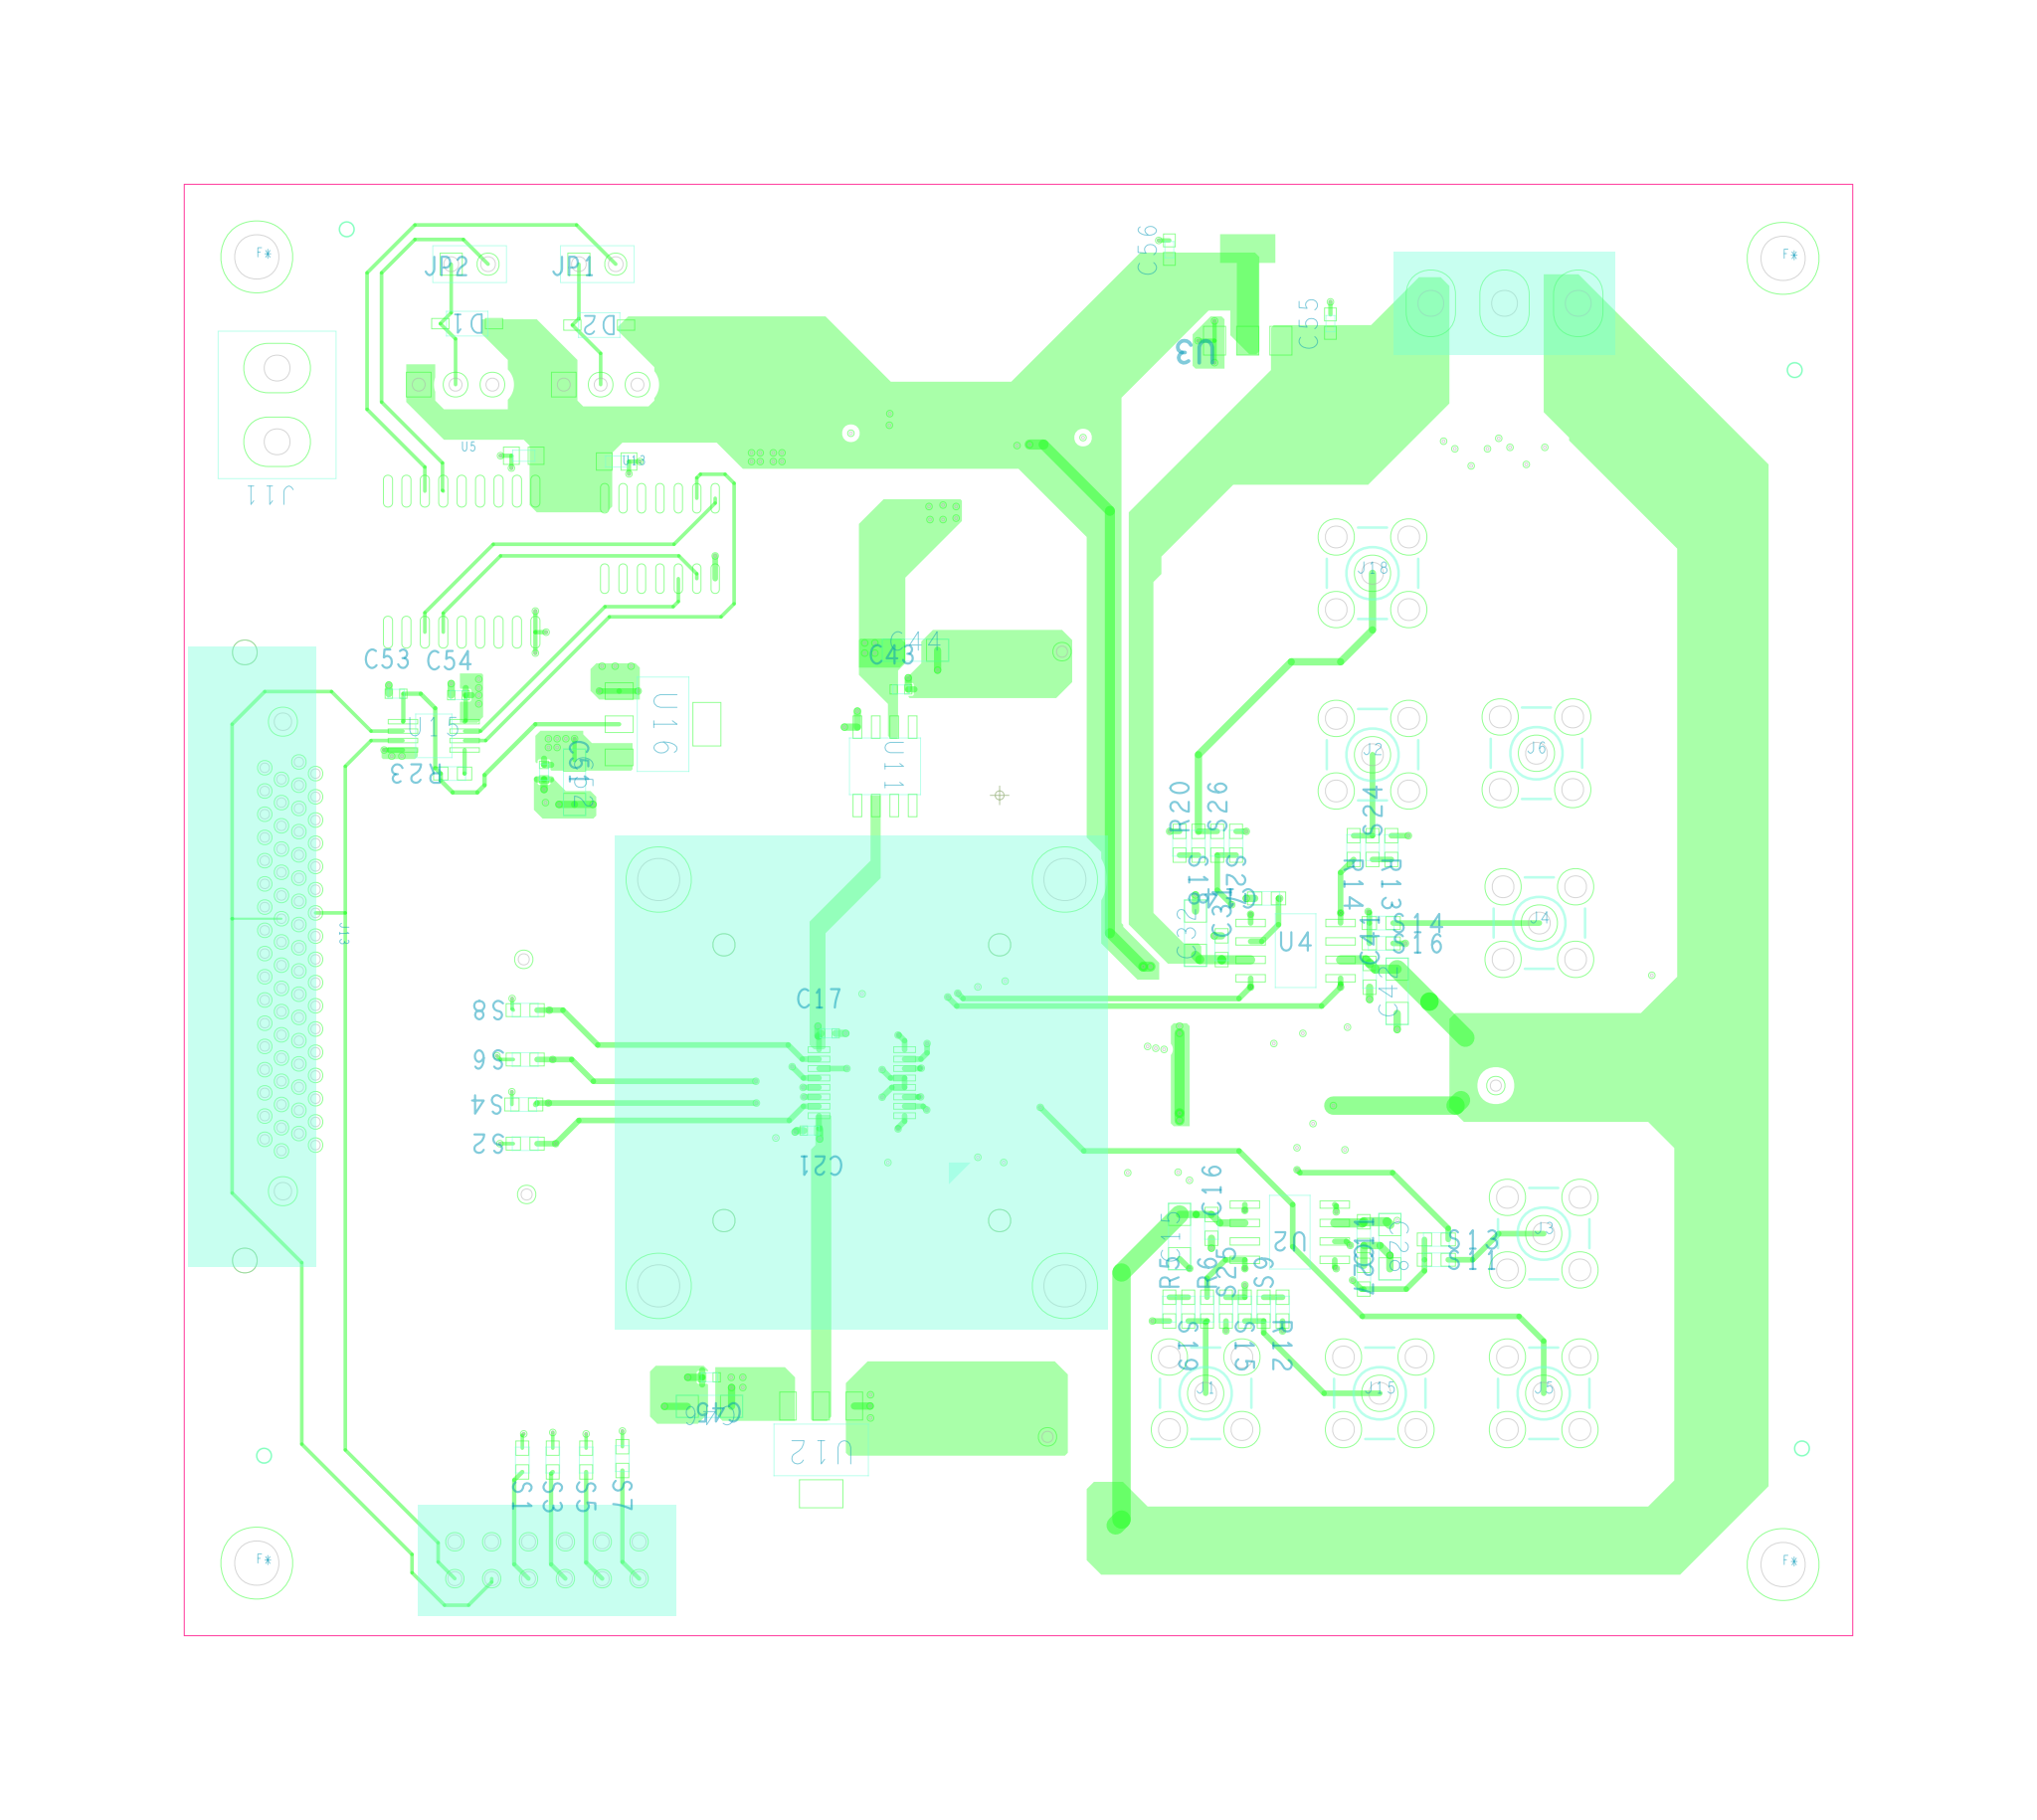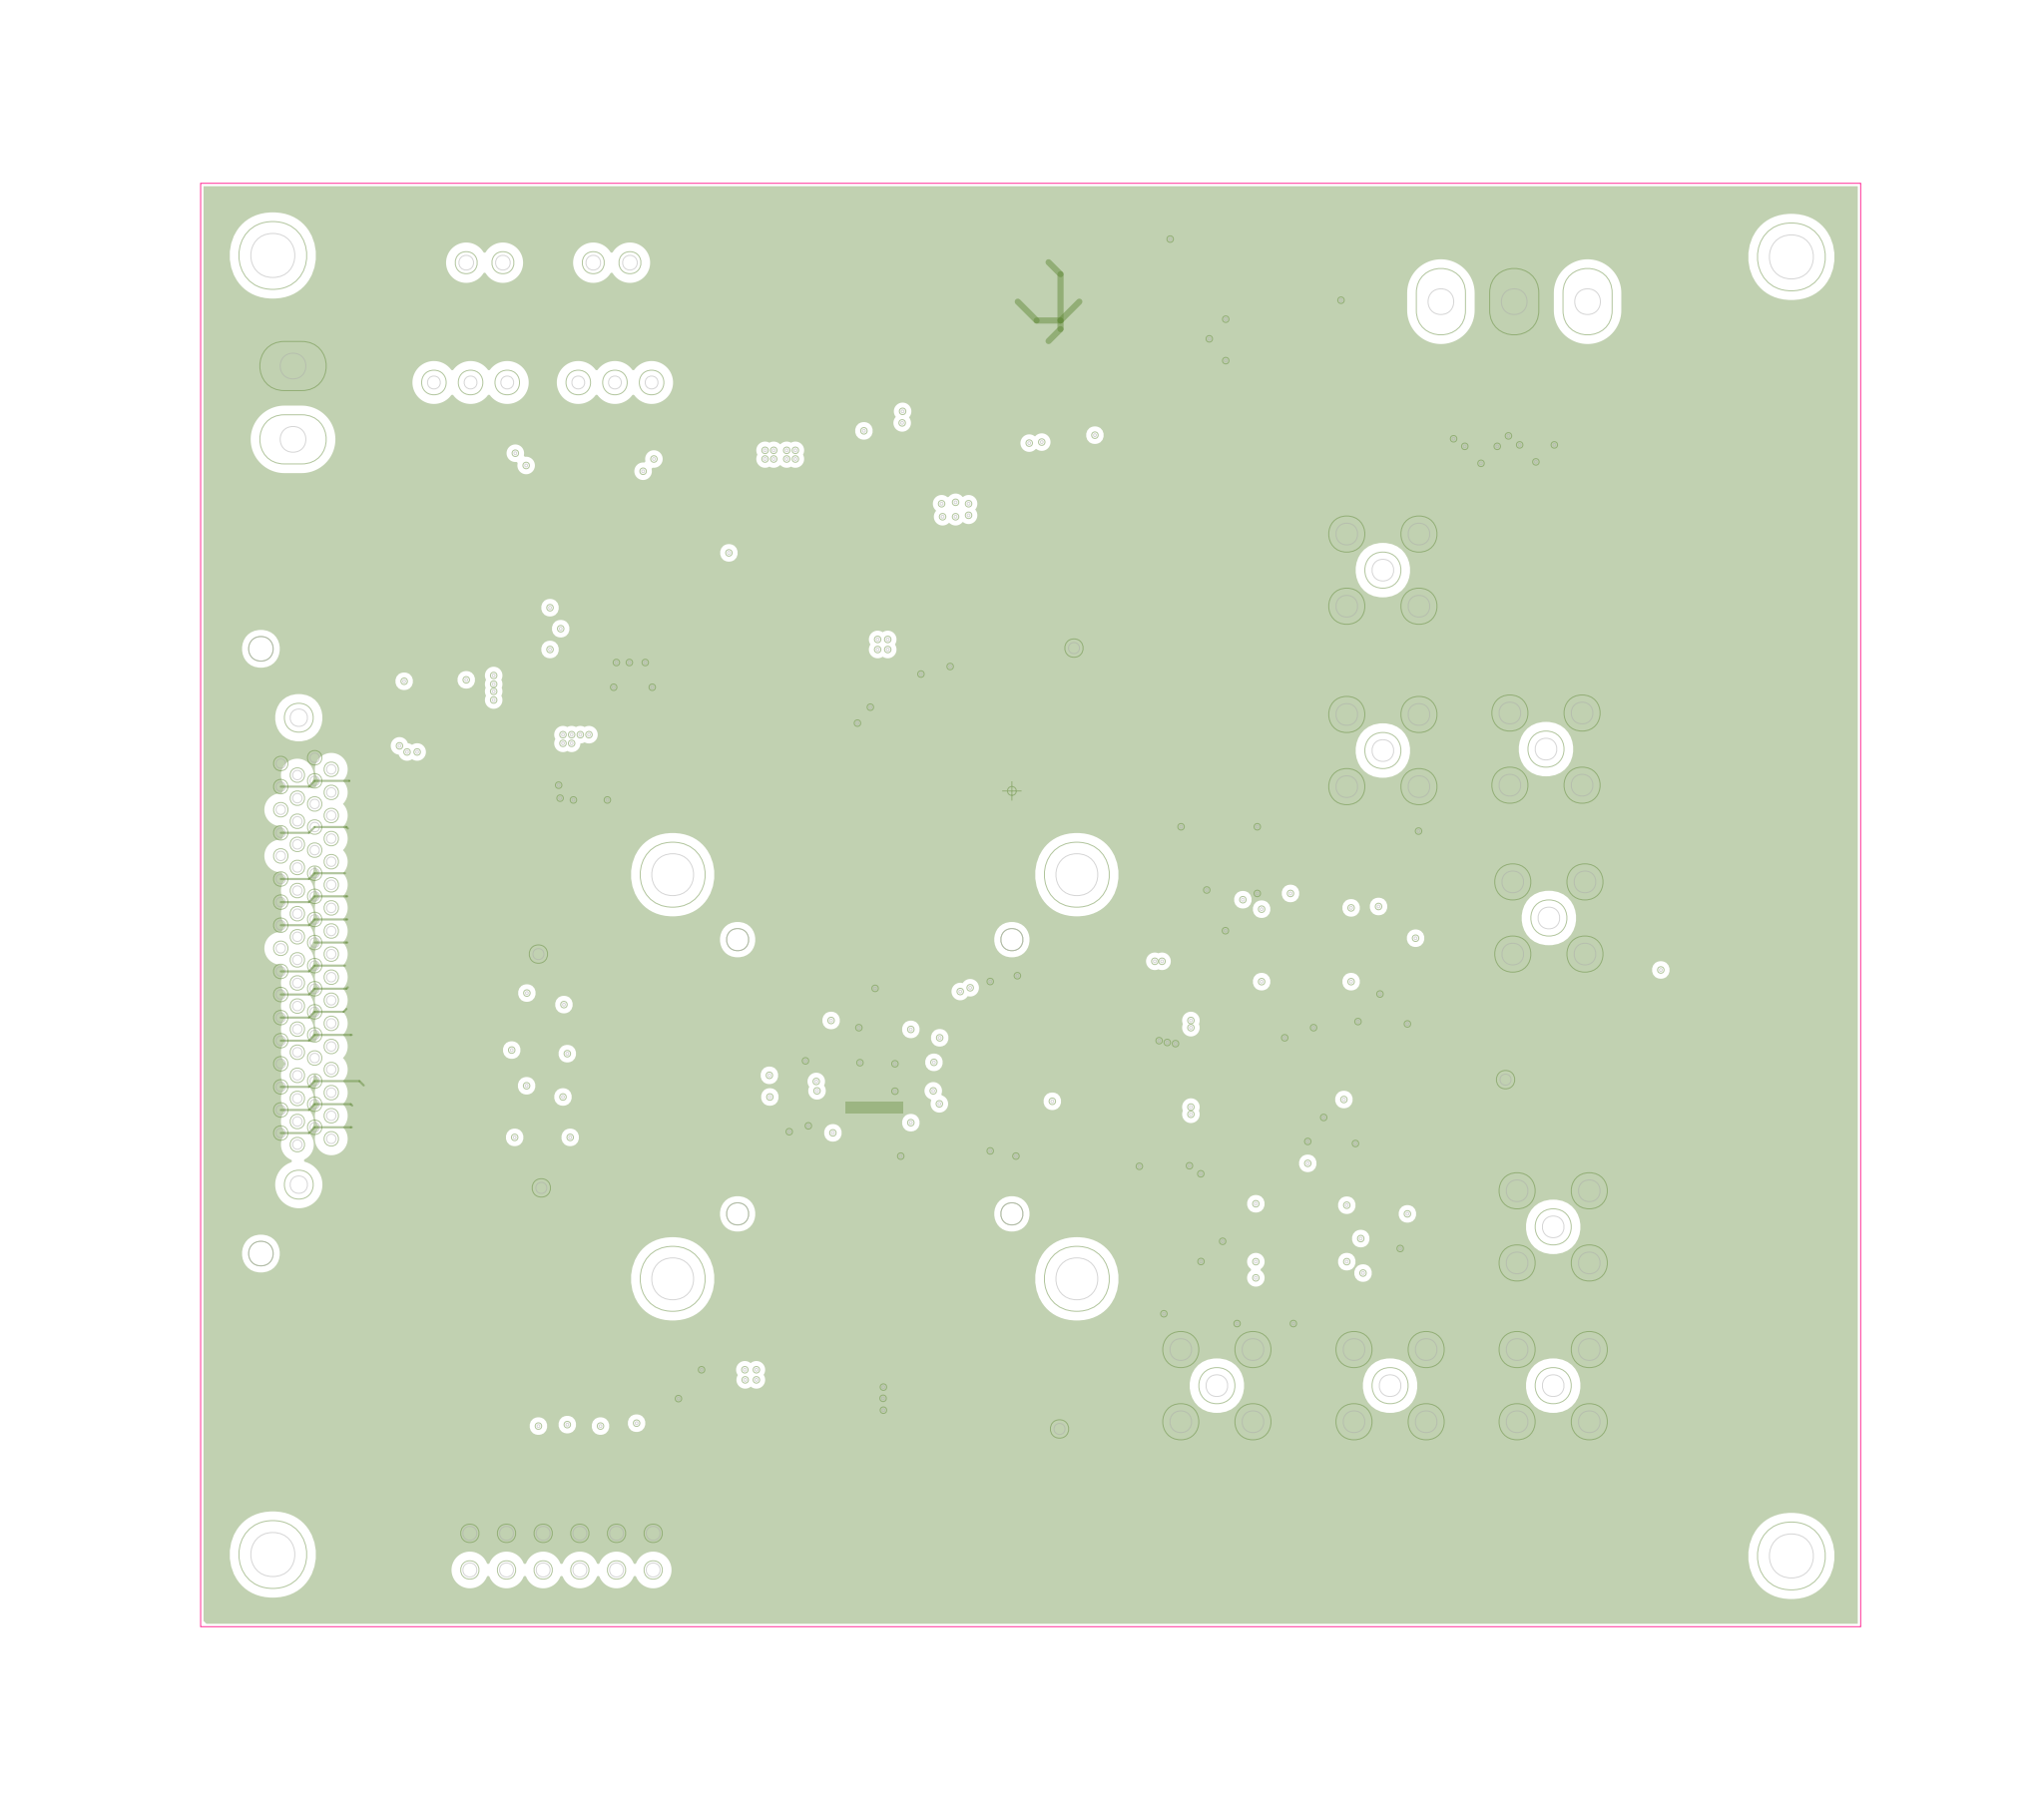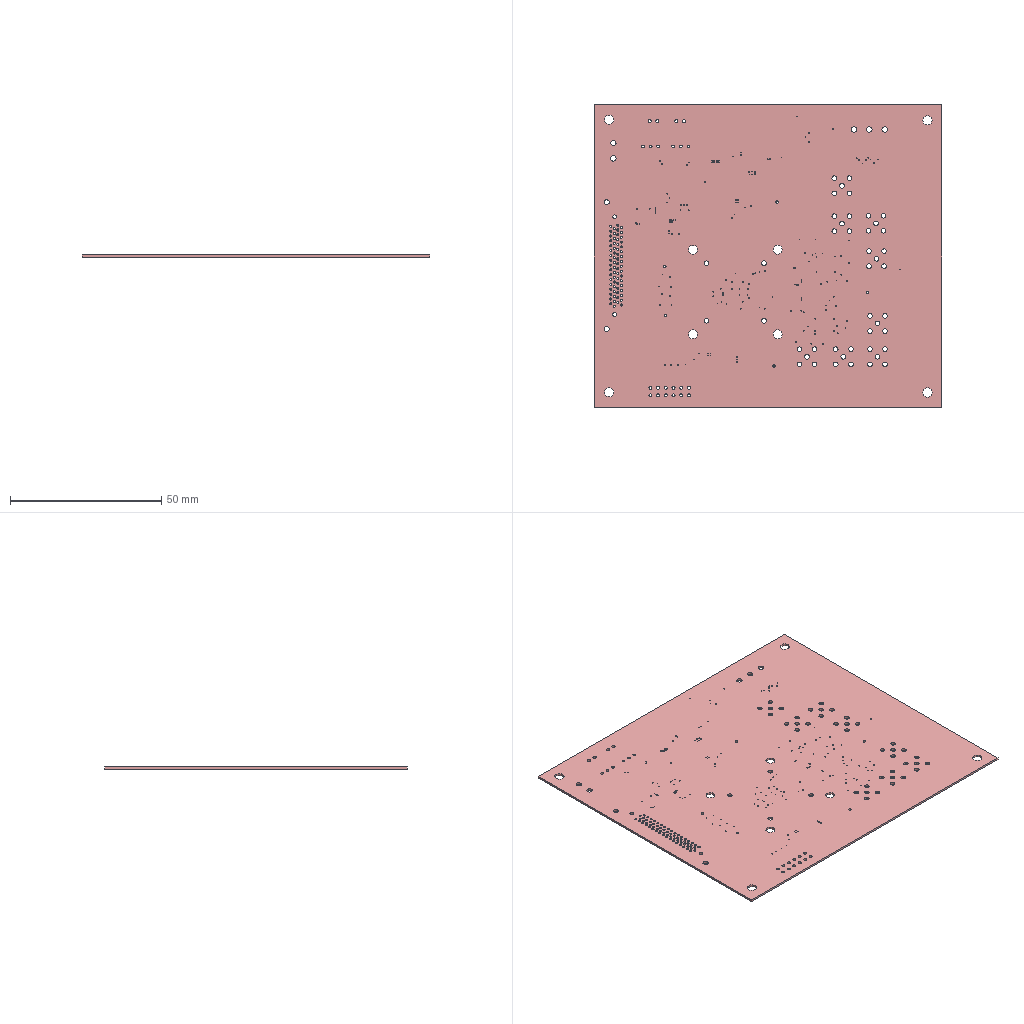Circuit board layout | Cadence Allegro | box 115 x 100 x 0.7 mm
Layer stack:
# Cadence Allegro layer stack of  (unit mm; from the constraint file cross-section; dielectric type: 0 not recorded (Allegro does not mark core vs prepreg), 3 surface material)
index,name,kind,layer,copper_thickness_mm,dielectric_type,dielectric_thickness_mm,dielectric_material,dielectric_constant
0,Top Surface,other,,,,,,
1,TOP,copper,TOP,0.0305,,,,
2,Dielectric1,dielectric,,,0,0.2032,FR-4,4.5
3,GND1,copper,GND1,0.0305,,,,
4,Dielectric2,dielectric,,,0,0.2032,FR-4,4.5
5,GND2,copper,GND2,0.0305,,,,
6,Dielectric3,dielectric,,,0,0.2032,FR-4,4.5
7,BOTTOM,copper,BOTTOM,0.0305,,,,
8,Bottom Surface,other,,,,,,
# drill layer pairs: low layer,high layer
drill_pair,TOP,BOTTOM
Part placement:
REFDES,COMP_VALUE,SYM_NAME,SYM_X,SYM_Y,SYM_ROTATE,SYM_MIRROR
AGND1,AGND1,TPC50D30,34.2,-20,0.000,NO
AGND2,AGND2,TPC50D30,4.3,9.9,0.000,NO
AGND3,AGND3,TPC50D30,3.3,-44.2,0.000,NO
C1,C,R0603,-7.7,-23.8,90.000,YES
C2,C,R0603,-4.2,-21.7,180.000,YES
C3,C,R0603,-4.2,-17.8,180.000,YES
C4,C,R0603,-7.7,-15.7,270.000,YES
C5,0.1UF,R0603,-7.4,-20.8,180.000,YES
C6,10UF,1206_C,-1.5,-22.3,90.000,YES
C7,10UF,1206_C,-1.5,-16.6,270.000,YES
C8,0.1UF,R0603,-7.4,-18.8,180.000,YES
C9,39PF,R0603,16.9,-30.2,90.000,YES
C10,39PF,R0603,23.2,-30.3,270.000,YES
C11,0.1UF,R0603,25.1,-33.2,90.000,NO
C12,39PF,R0603,23.5,-10.7,270.000,YES
C13,39PF,R0603,17.3,-10.8,90.000,YES
C14,0.1UF,R0603,18.4,-7.1,180.000,NO
C15,10UF,1206_C,12.4,-30.4,90.000,NO
C16,0.1UF,R0603,14.6,-29.7,90.000,NO
C17,0.1UF,0402,-11.8,-16.4,0.000,NO
C18,10UF,1206_C,-11,-14.8,180.000,YES
C19,0.1UF,R0603,1.1,-24.5,180.000,YES
C20,0.1UF,R0603,1.2,-14.2,0.000,YES
C21,0.1UF,0402,-13,-23.1,180.000,NO
C22,10UF,1206_C,-13.9,-24.8,0.000,YES
C23,0.1UF,R0603,20.9,-17.9,270.000,YES
C24,10UF,1206_C,23,-17.5,270.000,YES
C25,0.1UF,R0603,34.4,26.3,90.000,YES
C26,10UF,1206_C,36.3,25.5,90.000,YES
C27,0.1UF,R0603,25.1,-30.2,270.000,NO
C28,10UF,1206_C,26.9,-31.1,270.000,NO
C31,0.1UF,R0603,15.3,-10.5,90.000,NO
C32,10UF,1206_C,13.5,-9.5,90.000,NO
C35,0.1UF,R0603,30.6,26.1,90.000,YES
C36,10UF,1206_C,32.5,25.4,90.000,YES
C37,0.1UF,R0603,20.9,-21.8,270.000,YES
C38,10UF,1206_C,23,-22.9,270.000,YES
C41,0.1UF,R0603,25.5,-12.4,90.000,NO
C42,10UF,1206_C,27.4,-13.5,90.000,NO
C43,0.1UF,0402,-6.8,7.3,0.000,NO
C44,10UF,1206_C,-5.8,10,0.000,NO
C45,0.1UF,0402,-20,-40.1,180.000,NO
C46,10UF,1206_C,-20,-42.1,180.000,NO
C47,0.1uF,C0603,-26.4,23,180.000,NO
C48,0.1uF,C0603,-32.8,23.4,180.000,NO
C49,0.1uF,C0603,4.9,25.8,0.000,YES
C50,0.1uF,C0603,-9.4,26,180.000,YES
C51,0.1UF,0402,-31.4,1.6,270.000,NO
C52,10UF,1206_C,-29.3,0.9,270.000,NO
C53,0.1UF,0402,-41.6,7,0.000,NO
C54,0.1UF,0402,-37.3,6.9,0.000,NO
C55,1UF,C0402,22.8,32.5,90.000,NO
C56,4.7UF,C0402,11.7,37.6,90.000,NO
D1,1N4148,SOD_123,-36.7,32.5,180.000,NO
D2,1N4148,SOD_123,-27.6,32.4,180.000,NO
DGND1,DGND1,TPC50D30,-32.6,-27.5,0.000,NO
DGND2,DGND2,TPC50D30,-32.8,-11.3,0.000,NO
J1,VA,SMB_V-RJ45,14.2,-41.2,0.000,NO
J2,VB,SMB_V-RJ45,25.7,2.8,0.000,NO
J3,EXT COM A,SMB_V-RJ45,37.5,-30.2,0.000,NO
J4,EXT COM B,SMB_V-RJ45,37.2,-8.8,0.000,NO
J5,EXT REF A,SMB_V-RJ45,37.5,-41.2,0.000,NO
J6,EXT REF B,SMB_V-RJ45,37,2.9,0.000,NO
J11,REFA/B,POW2_BOLT,-49.8,26.9,180.000,NO
J13,VHDCI_68,VHDCI_68,-48.3,2.3,270.000,NO
J14,V+,POW3_BOLT,29.72,33.9,90.000,NO
J15,EXT COM A,SMB_V-RJ45,26.2,-41.2,0.000,NO
J17,CON6,CON6X2,-24.85,-53.97,270.000,NO
J18,EXT REF B,SMB_V-RJ45,25.7,15.3,0.000,NO
JP1,con2/,HDR_1X2,-29,36.6,0.000,NO
JP2,con2/,HDR_1X2,-37.8,36.6,0.000,NO
LK1,conv1x3,HDR254M-1X3,-30.04,28.3,0.000,NO
LK2,conv1x3,HDR254M-1X3,-40.04,28.3,0.000,NO
R1,33r,R0603,-6.3,-23.8,270.000,YES
R2,33r,R0603,-4.2,-23.1,0.000,YES
R3,33r,R0603,-4.2,-16.4,0.000,YES
R4,33r,R0603,-6.3,-15.7,90.000,YES
R5,49.9r,R0603,11.7,-35.4,90.000,NO
R6,499r,R0603,14.3,-35.4,90.000,NO
R7,499r,R0603,18.5,-30.2,270.000,YES
R8,499r,R0603,21.6,-30.3,270.000,YES
R9,523r,R0603,20.1,-32,270.000,YES
R10,10K,R0603,18.3,-25.1,270.000,YES
R11,10K,R0603,19.7,-25.1,90.000,YES
R12,49.9r,R0603,19.5,-35.4,270.000,NO
R13,49.9r,R0603,27,-3.6,270.000,NO
R14,499r,R0603,24.4,-3.6,270.000,NO
R15,499r,R0603,21.9,-10.7,90.000,YES
R16,523r,R0603,16,-9.2,90.000,YES
R17,499r,R0603,18.9,-10.8,270.000,YES
R18,10K,R0603,17.5,-15.5,90.000,YES
R19,10K,R0603,18.9,-15.5,270.000,YES
R20,49.9r,R0603,12.4,-3.3,90.000,NO
R21,0,R0603,-15.1,-21.2,180.000,YES
R22,0,R0603,-15.1,-19.7,0.000,YES
R23,0,R0603,-37.7,1.5,180.000,NO
S1,S,R0603,-32.9,-45.8,270.000,NO
S2,S,R0603,-32.7,-24,180.000,NO
S3,S,R0603,-30.8,-45.8,270.000,NO
S4,S,R0603,-32.8,-21.3,180.000,NO
S5,S,R0603,-28.5,-45.8,270.000,NO
S6,S,R0603,-32.7,-18.2,180.000,NO
S7,S,R0603,-26,-45.7,270.000,NO
S8,S,R0603,-32.7,-14.8,180.000,NO
S9,S,R0603,18.2,-35.4,90.000,NO
S11,S,R0603,30.1,-32,0.000,NO
S13,S,R0603,30.1,-30.6,0.000,NO
S14,S,R0603,26.3,-8.8,0.000,NO
S15,S,R0603,16.9,-35.4,270.000,NO
S16,S,R0603,26.3,-10.2,0.000,NO
S18,S,R0603,13.7,-3.3,270.000,NO
S19,S,R0603,13,-35.4,270.000,NO
S20,S,R0603,1.1,-21.7,0.000,YES
S21,S,R0603,1.1,-23.1,0.000,YES
S22,S,R0603,1.2,-17,0.000,YES
S23,S,R0603,1.2,-15.6,0.000,YES
S24,S,R0603,25.7,-3.6,90.000,NO
S25,S,R0603,15.6,-35.4,90.000,NO
S26,S,R0603,15,-3.3,90.000,NO
S27,S,R0603,16.3,-3.3,270.000,NO
U1,AD7356,AD7356CHAZUO,-9.5,-19.8,180.000,NO
U2,AD8138,SOIC8_TB,20,-30.1,180.000,NO
U3,LDL1117-5,SOT-223,14.814,31.325,180.000,NO
U4,AD8138,SOIC8_TB,20.4,-10.7,0.000,NO
U5,ULN2803,ULN2803,-37.078,16.1,0.000,NO
U6,ADR421,SOIC8_TB,7.1,-24.1,0.000,YES
U7,ADR421,SOIC8_TB,7.1,-14.9,0.000,YES
U8,AD8022ARM,MSOP_8,18,-20.4,270.000,YES
U10,UB2_DIP,UB2_DIP,4.2,29.6,0.000,YES
U11,ADR431ARZ,SOIC-8,-7.9,2,270.000,NO
U12,ADP3338AKCZ-3.3,SOT223-2,-12.3,-45.1,180.000,NO
U13,74HC14,74HC14,-23.414,17.7,0.000,NO
U14,UB2_DIP,UB2_DIP,-8.3,29.6,0.000,YES
U15,SN74LVC2T45,SOP8_DCT,-39,4.1,0.000,NO
U16,ADP3338AKCZ-3.3,SOT223-2,-23.2,4.9,270.000,NO
Pad and via stacks:
# Allegro (Cadence) via spans and padstacks; design units: ("millimeters" 4 10000)
# via spans: padstack,start_layer,end_layer,net_example,count
3-TOP-BOTTOM,ETCH/TOP,ETCH/BOTTOM,GND,173
# Allegro padstack definitions: name,start_layer,end_layer,drill,plating,holeType,type
43X47,"ETCH/TOP","ETCH/TOP",0.0,"NON_PLATED","none","smd"
SMD60SQ,"ETCH/TOP","ETCH/TOP",0.0,"PLATED","none","smd"
39X35,"ETCH/TOP","ETCH/TOP",0.0,"PLATED","none","smd"
R60_16,"ETCH/TOP","ETCH/TOP",0.0,"PLATED","none","smd"
SMD_80_20_REC,"ETCH/TOP","ETCH/TOP",0.0,"PLATED","none","smd"
R58_15,"ETCH/TOP","ETCH/TOP",0.0,"PLATED","none","smd"
THC2_5D1_5,"ETCH/TOP","ETCH/BOTTOM",1.5,"PLATED","circle_drill","through"
PAD40CIR32D_TB,"ETCH/TOP","ETCH/BOTTOM",0.8128,"PLATED","circle_drill","through"
PAD_POW_70_TB,"ETCH/TOP","ETCH/BOTTOM",1.778,"PLATED","circle_drill","through"
VIA,"ETCH/TOP","ETCH/BOTTOM",0.3302,"PLATED","circle_drill","through"
VIA0_8MM,"ETCH/TOP","ETCH/BOTTOM",0.8,"PLATED","circle_drill","through"
2,"ETCH/TOP","ETCH/BOTTOM",0.8,"PLATED","circle_drill","through"
VIA0R2_0R45,"ETCH/TOP","ETCH/BOTTOM",0.2,"PLATED","circle_drill","through"
3-TOP-BOTTOM,"ETCH/TOP","ETCH/BOTTOM",0.2,"PLATED","circle_drill","through"
VIA4020,"ETCH/TOP","ETCH/BOTTOM",0.508,"PLATED","circle_drill","through"
4-TOP-BOTTOM,"ETCH/TOP","ETCH/BOTTOM",0.508,"PLATED","circle_drill","through"
27_6MIL,"ETCH/TOP","ETCH/BOTTOM",0.7112,"PLATED","circle_drill","through"
HOLE3MM6,"ETCH/TOP","ETCH/BOTTOM",1.6,"NON_PLATED","circle_drill","through"
PAD60CIR35D_TB,"ETCH/TOP","ETCH/BOTTOM",0.889,"PLATED","circle_drill","through"
PAD87CIR67D-F,"ETCH/TOP","ETCH/BOTTOM",1.702,"PLATED","circle_drill","through"
BALL71,"ETCH/TOP","ETCH/TOP",0.0,"PLATED","none","smd"
1_75X0,"ETCH/TOP","ETCH/TOP",0.0,"NON_PLATED","none","smd"
PAD195CIR120D_TB,"ETCH/TOP","ETCH/BOTTOM",3.048,"PLATED","circle_drill","through"
THC5_3D3_3,"ETCH/TOP","ETCH/BOTTOM",3.3,"PLATED","circle_drill","through"
C50D30,"ETCH/TOP","ETCH/BOTTOM",0.762,"PLATED","circle_drill","through"
0_3X1_0MM,"ETCH/TOP","ETCH/TOP",0.0,"NON_PLATED","none","smd"
DRILL_1_6MM,"ETCH/TOP","ETCH/BOTTOM",1.6,"PLATED","circle_drill","through"
DRILL_3MM2,"ETCH/TOP","ETCH/BOTTOM",3.0,"PLATED","circle_drill","through"
DRILL_2_9MM,"ETCH/TOP","ETCH/BOTTOM",2.9,"PLATED","circle_drill","through"
DRILL_1_53MM,"ETCH/TOP","ETCH/BOTTOM",1.53,"PLATED","circle_drill","through"
SMD1_5X0_4MM,"ETCH/TOP","ETCH/TOP",0.0,"NON_PLATED","none","smd"
PAD50CIR38D,"ETCH/TOP","ETCH/BOTTOM",0.9652,"PLATED","circle_drill","through"
SMD_100_30_REC,"ETCH/TOP","ETCH/TOP",0.0,"PLATED","none","smd"
HOLE105CIR95_LRC,"ETCH/TOP","ETCH/BOTTOM",2.413,"NON_PLATED","circle_drill","through"
HOLE62_LRC,"ETCH/TOP","ETCH/BOTTOM",1.575,"NON_PLATED","circle_drill","through"
R20_25,"ETCH/TOP","ETCH/TOP",0.0,"NON_PLATED","none","smd"
TH35_C67-2,"ETCH/TOP","ETCH/BOTTOM",0.889,"PLATED","circle_drill","through"
TH35_SQ67-2,"ETCH/TOP","ETCH/BOTTOM",0.889,"PLATED","circle_drill","through"
R47_28,"ETCH/TOP","ETCH/TOP",0.0,"NON_PLATED","none","smd"
S60H40,"ETCH/TOP","ETCH/BOTTOM",1.016,"PLATED","circle_drill","through"
C60H40,"ETCH/TOP","ETCH/BOTTOM",1.016,"PLATED","circle_drill","through"
SMD_R472X1221P0S40,"ETCH/TOP","ETCH/TOP",0.0,"NON_PLATED","none","smd"
SMD1_55X0_6,"ETCH/TOP","ETCH/TOP",0.0,"PLATED","none","smd"
76X118,"ETCH/TOP","ETCH/TOP",0.0,"NON_PLATED","none","smd"
45X76,"ETCH/TOP","ETCH/TOP",0.0,"NON_PLATED","none","smd"
SMD_O226X802P0S40,"ETCH/TOP","ETCH/TOP",0.0,"NON_PLATED","none","smd"
SMD_O248X866P0S40,"ETCH/TOP","ETCH/TOP",0.0,"NON_PLATED","none","smd"
PAD0R65_1R0_CIR,"ETCH/TOP","ETCH/BOTTOM",0.65,"PLATED","circle_drill","through"
HOLE1-7CIR,"ETCH/TOP","ETCH/BOTTOM",1.7,"PLATED","circle_drill","through"
PAD1-2_2-0_CIR,"ETCH/TOP","ETCH/BOTTOM",1.2,"PLATED","circle_drill","through"
PSM_FID_130SM,"ETCH/TOP","ETCH/TOP",0.0,"NON_PLATED","none","smd"
35X32,"ETCH/TOP","ETCH/TOP",0.0,"NON_PLATED","none","smd"
SMD_R780X600P0S40,"ETCH/TOP","ETCH/TOP",0.0,"NON_PLATED","none","smd"
SMD_80_12_REC,"ETCH/TOP","ETCH/TOP",0.0,"PLATED","none","smd"
Design rules, without the lines most boards share, first 14 of 28 lines:
# Cadence Allegro design rules of  (from the Constraint Manager export constraints.dcfx, design unit mm; typed fields in mm)
# columns: name | kind | enabled | priority | scope1 | scope2 | descriptor | typed fields (field=value)
# Allegro precedence (priority 1 wins): 1 Region class-to-class, 2 Region class, 3 Region, 4 class-to-class, 5 DiffPair/Bus/NetGroup override, 6 NetClass, 7 constraint set (CSet) default
# per-layer values are written LAYER=value in the descriptor and LAYER:mm in the typed field; a maximum of 0 means no limit set
# --- net classes (and buses / net groups) ---
S | Bus | enabled | 5 | S<0>, S<1> | All | Bus (members: 2 Net) |
# --- track widths, neck and differential-pair gap (physical constraint sets) ---
DEFAULT | PhysicalCSet | enabled | 7 | Design default | All | Physical Constraint (Min Line Width=0.127mm) (Max Line Width=0mm) (Min Neck Width=0.127mm) (Max Neck Length=0mm) (DiffPair Primary Gap=0mm) (DiffPair Neck Gap=0mm) (DiffPair Min Space=0mm) (DiffPair Coupled +Tol=0mm) (DiffPair Coupled -Tol=0mm) (Min BB Via Stagger=0.127mm) (Max BB Via Stagger=0mm) (T-junctions=ANYWHERE) (Pad-pad direct connect=ALL_ALLOWED) (Allowed vias=TOP-BOTTOM, 1-TOP-BOTTOM, 3-TOP-BOTTOM, 4-TOP-BOTTOM) | min_line_width=0.127 min_neck_width=0.127 min_bvia_stagger=0.127 max_bvia_stagger=0 ts_allowed=ANYWHERE diffp_primary_gap=0 diffp_neck_gap=0 max_line_width=0 maximum_neck_length=0 pad_pad_direct_connect=ALL_ALLOWED allow_on_etch_subclass=TRUE diffp_coupled_plus=0 diffp_coupled_minus=0 diffp_min_space=0 vias=TOP-BOTTOM,1-TOP-BOTTOM,3-TOP-BOTTOM,4-TOP-BOTTOM
# --- clearances: line / pad / via / shape / hole (spacing constraint sets) ---
DEFAULT | SpacingCSet | enabled | 7 | Design default | All | Clearance Constraint (Line-Line=0.127mm) (Line-SMD Pad=0.2032mm) (Line-Thru Pin=0.2032mm) (Line-Via=0.127mm) (Line-Shape=0.3mm) (SMD Pad-SMD Pad=0.2032mm) (Thru Pin-Thru Pin=0.2032mm) (Thru Pin-SMD Pad=0.2032mm) (SMD Pad-Via=0.127mm) (Thru Pin-Via=0.2032mm) (Via-Via=0.127mm) (Shape-SMD Pad=0.2mm) (Shape-Thru Pin=0.381mm) (Shape-Via=0.381mm) (Shape-Shape=0.381mm) (Hole-Hole=0.2032mm) (Hole-Line=0.2032mm) (Hole-Shape=0.2032mm) (BB Via-BB Via=0.127mm) (uVia-uVia=0.127mm) | line_to_line_spacing=0.127 line_to_smdpin_spacing=0.2032 smdpin_to_smdpin_spacing=0.2032 line_to_testpin_spacing=0.2032 testpin_to_thrupin_spacing=0.2032 testpin_to_testpin_spacing=0.2032 line_to_thruvia_spacing=0.127 smdpin_to_thruvia_spacing=0.127 testpin_to_thruvia_spacing=0.127 thruvia_to_thruvia_spacing=0.127 bbv_to_line_spacing=0.127 bbv_to_thrupin_spacing=0.2032 bbv_to_smdpin_spacing=0.127 bbv_to_testpin_spacing=0.127 bbv_to_bbv_spacing=0.127 line_to_testvia_spacing=0.127 smdpin_to_testvia_spacing=0.127 testpin_to_testvia_spacing=0.127 testvia_to_thruvia_spacing=0.127 bbv_to_testvia_spacing=0.127 testvia_to_testvia_spacing=0.127 mvia_to_line_spacing=0.127 mvia_to_thrupin_spacing=0.127 mvia_to_smdpin_spacing=0.127 mvia_to_testpin_spacing=0.127 mvia_to_thruvia_spacing=0.127 mvia_to_bbv_spacing=0.127 mvia_to_mvia_spacing=0.127 line_to_shape_spacing=0.3 shape_to_smdpin_spacing=0.2 shape_to_testpin_spacing=0.381 shape_to_thruvia_spacing=0.381 bbv_to_shape_spacing=0.381 shape_to_testvia_spacing=0.381 mvia_to_shape_spacing=0.127 shape_to_shape_spacing=0.381 bondpad_to_line_spacing=0.127 thrupin_to_bondpad_spacing=0.2032 smdpin_to_bondpad_spacing=0.127 bondpad_to_testpin_spacing=0.127 bondpad_to_thruvia_spacing=0.127 bondpad_to_bbv_spacing=0.127 bondpad_to_testvia_spacing=0.127 bondpad_to_mvia_spacing=0.127 bondpad_to_bondpad_spacing=0.127 thrupin_to_thrupin_spacing=0.2032 thrupin_to_smdpin_spacing=0.2032 thrupin_to_thruvia_spacing=0.2032 line_to_thrupin_spacing=0.2032 thrupin_to_shape_spacing=0.381 bbv_to_thruvia_spacing=0.127 smdpin_to_testpin_spacing=0.2032 testvia_to_thrupin_spacing=0.2032 bondpad_to_shape_spacing=0.381 hole_to_pin_spacing=0.2032 hole_to_via_spacing=0.2032 hole_to_line_spacing=0.2032 hole_to_shape_spacing=0.2032 hole_to_hole_spacing=0.2032 mvia_to_testvia_spacing=0.127 bondpad_to_bondpad_diffp_spc=0.127 min_bvia_gap=0.127
DEFAULT | SameNetSpacingCSet | enabled | 7 | Design default | All | Same-Net Clearance (Line-Line=0.127mm) (Line-SMD Pad=0.127mm) (Line-Thru Pin=0.127mm) (Line-Via=0.127mm) (Line-Shape=0.127mm) (SMD Pad-SMD Pad=0.127mm) (Thru Pin-Thru Pin=0.127mm) (Thru Pin-SMD Pad=0.127mm) (SMD Pad-Via=0.127mm) (Thru Pin-Via=0.127mm) (Via-Via=0.127mm) (Shape-SMD Pad=0.127mm) (Shape-Thru Pin=0.127mm) (Shape-Via=0.127mm) (Shape-Shape=0.127mm) (Hole-Hole=0.2032mm) (Hole-Line=0.2032mm) (Hole-Shape=0.2032mm) (BB Via-BB Via=0.127mm) (uVia-uVia=0.127mm) | sn_thrupin_to_thrupin_spacing=0.127 sn_thrupin_to_smdpin_spacing=0.127 sn_thrupin_to_thruvia_spacing=0.127 sn_line_to_thrupin_spacing=0.127 sn_thrupin_to_shape_spacing=0.127 sn_smdpin_to_smdpin_spacing=0.127 sn_smdpin_to_thruvia_spacing=0.127 sn_line_to_smdpin_spacing=0.127 sn_shape_to_smdpin_spacing=0.127 sn_thruvia_to_thruvia_spacing=0.127 sn_line_to_thruvia_spacing=0.127 sn_shape_to_thruvia_spacing=0.127 sn_line_to_line_spacing=0.127 sn_line_to_shape_spacing=0.127 sn_shape_to_shape_spacing=0.127 sn_bbv_to_bbv_spacing=0.127 sn_bbv_to_thrupin_spacing=0.127 sn_bbv_to_smdpin_spacing=0.127 sn_bbv_to_thruvia_spacing=0.127 sn_bbv_to_line_spacing=0.127 sn_bbv_to_shape_spacing=0.127 sn_bbv_to_testpin_spacing=0.127 sn_bbv_to_testvia_spacing=0.127 sn_testpin_to_testpin_spacing=0.127 sn_testpin_to_thrupin_spacing=0.127 sn_smdpin_to_testpin_spacing=0.127 sn_testpin_to_thruvia_spacing=0.127 sn_testpin_to_testvia_spacing=0.127 sn_line_to_testpin_spacing=0.127 sn_shape_to_testpin_spacing=0.127 sn_testvia_to_testvia_spacing=0.127 sn_testvia_to_thrupin_spacing=0.127 sn_smdpin_to_testvia_spacing=0.127 sn_testvia_to_thruvia_spacing=0.127 sn_line_to_testvia_spacing=0.127 sn_shape_to_testvia_spacing=0.127 sn_bondpad_to_bondpad_spacing=0.127 sn_thrupin_to_bondpad_spacing=0.127 sn_smdpin_to_bondpad_spacing=0.127 sn_bondpad_to_thruvia_spacing=0.127 sn_bondpad_to_line_spacing=0.127 sn_bondpad_to_shape_spacing=0.127 sn_bondpad_to_bbv_spacing=0.127 sn_bondpad_to_testpin_spacing=0.127 sn_bondpad_to_testvia_spacing=0.127 same_net=TRUE sn_hole_to_pin_spacing=0.2032 sn_hole_to_via_spacing=0.2032 sn_hole_to_line_spacing=0.2032 sn_hole_to_shape_spacing=0.2032 sn_hole_to_hole_spacing=0.2032 sn_mvia_to_mvia_spacing=0.127 sn_mvia_to_thrupin_spacing=0.127 sn_mvia_to_smdpin_spacing=0.127 sn_mvia_to_thruvia_spacing=0.127 sn_mvia_to_bbv_spacing=0.127 sn_mvia_to_line_spacing=0.127 sn_mvia_to_shape_spacing=0.127 sn_mvia_to_testpin_spacing=0.127 sn_mvia_to_testvia_spacing=0.127 sn_bondpad_to_mvia_spacing=0.127
# --- differential pairs (2) ---
VINB | DiffPair | enabled | 5 | VINB+ | VINB- | Differential Pair (Primary Gap=0mm) (Min Line Width=0.127mm) (Physical CSet=DEFAULT) | gap=0 width=0.127
VINA | DiffPair | enabled | 5 | VINA+ | VINA- | Differential Pair (Primary Gap=0mm) (Min Line Width=0.127mm) (Physical CSet=DEFAULT) | gap=0 width=0.127